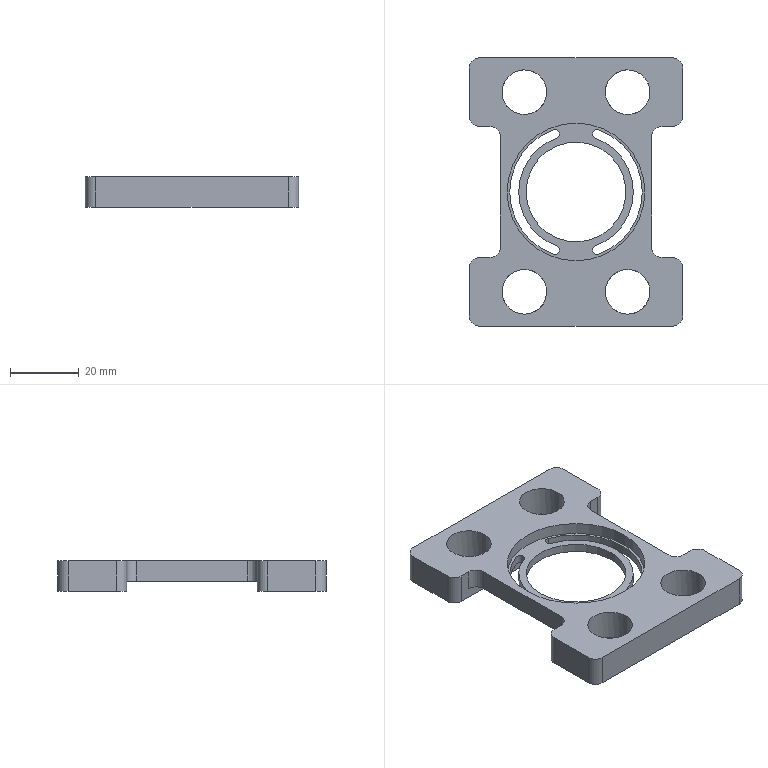NC program | NX | posted with a generic post | part box 62 x 78 x 9 mm
Lines 1 to 792 of 3044:
N10 G17 G21 G94 G90
(FLOOR_WALL , TOOL : D10)
N12 T10 M6
N14 G54
N16 G17 G0 G90 X-49. Y32.997 S9500 M3
N18 G43 Z30. H10
N20 Z3.
N22 G94 G1 Z0. F1250.
N24 X-46.
N26 X46.
N28 Y28.228
N30 X-46.
N32 Y23.459
N34 X46.
N36 Y18.69
N38 X-46.
N40 Y13.921
N42 X46.
N44 Y9.152
N46 X-46.
N48 Y4.383
N50 X46.
N52 Y-0.386
N54 X-46.
N56 Y-5.155
N58 X46.
N60 Y-9.924
N62 X-46.
N64 Y-14.693
N66 X46.
N68 Y-19.462
N70 X-46.
N72 Y-24.231
N74 X46.
N76 Y-29.
N78 X-46.
N80 X-49.
N82 Z3.
N84 G0 Z30.
(HOLE_MILLING , TOOL : D10)
N86 X-29. Y15.
N88 Z0.5
N90 G3 X-29.7 Y14.3 R0.7
N92 X-29. Y13.6 R0.7
N94 X-29. Y13.6 Z0. I0. J1.4
N96 X-29. Y13.6 Z-0.5 I0. J1.4
N98 X-29. Y13.6 Z-1. I0. J1.4
N100 X-29. Y13.6 Z-1.5 I0. J1.4
N102 X-29. Y13.6 Z-2. I0. J1.4
N104 X-29. Y13.6 Z-2.5 I0. J1.4
N106 X-29. Y13.6 Z-3. I0. J1.4
N108 X-29. Y13.6 Z-3.5 I0. J1.4
N110 X-29. Y13.6 Z-4. I0. J1.4
N112 X-29. Y13.6 Z-4.5 I0. J1.4
N114 X-29. Y13.6 Z-5. I0. J1.4
N116 X-29. Y13.6 Z-5.5 I0. J1.4
N118 X-29. Y13.6 Z-6. I0. J1.4
N120 X-29. Y13.6 Z-6.5 I0. J1.4
N122 X-29. Y13.6 Z-7. I0. J1.4
N124 X-29. Y13.6 Z-7.5 I0. J1.4
N126 X-29. Y13.6 Z-8. I0. J1.4
N128 X-29. Y13.6 Z-8.5 I0. J1.4
N130 X-29. Y13.6 Z-9. I0. J1.4
N132 X-27.6 Y15. R1.4
N134 X-29. Y13.6 R-1.4
N136 X-28.3 Y14.3 R0.7
N138 X-29. Y15. R0.7
N140 G0 Z30.
N142 Y-15.
N144 Z0.5
N146 G3 X-29.7 Y-15.7 R0.7
N148 X-29. Y-16.4 R0.7
N150 X-29. Y-16.4 Z0. I0. J1.4
N152 X-29. Y-16.4 Z-0.5 I0. J1.4
N154 X-29. Y-16.4 Z-1. I0. J1.4
N156 X-29. Y-16.4 Z-1.5 I0. J1.4
N158 X-29. Y-16.4 Z-2. I0. J1.4
N160 X-29. Y-16.4 Z-2.5 I0. J1.4
N162 X-29. Y-16.4 Z-3. I0. J1.4
N164 X-29. Y-16.4 Z-3.5 I0. J1.4
N166 X-29. Y-16.4 Z-4. I0. J1.4
N168 X-29. Y-16.4 Z-4.5 I0. J1.4
N170 X-29. Y-16.4 Z-5. I0. J1.4
N172 X-29. Y-16.4 Z-5.5 I0. J1.4
N174 X-29. Y-16.4 Z-6. I0. J1.4
N176 X-29. Y-16.4 Z-6.5 I0. J1.4
N178 X-29. Y-16.4 Z-7. I0. J1.4
N180 X-29. Y-16.4 Z-7.5 I0. J1.4
N182 X-29. Y-16.4 Z-8. I0. J1.4
N184 X-29. Y-16.4 Z-8.5 I0. J1.4
N186 X-29. Y-16.4 Z-9. I0. J1.4
N188 X-27.6 Y-15. R1.4
N190 X-29. Y-16.4 R-1.4
N192 X-28.3 Y-15.7 R0.7
N194 X-29. Y-15. R0.7
N196 G0 Z30.
N198 X29.
N200 Z0.5
N202 G3 X28.3 Y-15.7 R0.7
N204 X29. Y-16.4 R0.7
N206 X29. Y-16.4 Z0. I0. J1.4
N208 X29. Y-16.4 Z-0.5 I0. J1.4
N210 X29. Y-16.4 Z-1. I0. J1.4
N212 X29. Y-16.4 Z-1.5 I0. J1.4
N214 X29. Y-16.4 Z-2. I0. J1.4
N216 X29. Y-16.4 Z-2.5 I0. J1.4
N218 X29. Y-16.4 Z-3. I0. J1.4
N220 X29. Y-16.4 Z-3.5 I0. J1.4
N222 X29. Y-16.4 Z-4. I0. J1.4
N224 X29. Y-16.4 Z-4.5 I0. J1.4
N226 X29. Y-16.4 Z-5. I0. J1.4
N228 X29. Y-16.4 Z-5.5 I0. J1.4
N230 X29. Y-16.4 Z-6. I0. J1.4
N232 X29. Y-16.4 Z-6.5 I0. J1.4
N234 X29. Y-16.4 Z-7. I0. J1.4
N236 X29. Y-16.4 Z-7.5 I0. J1.4
N238 X29. Y-16.4 Z-8. I0. J1.4
N240 X29. Y-16.4 Z-8.5 I0. J1.4
N242 X29. Y-16.4 Z-9. I0. J1.4
N244 X30.4 Y-15. R1.4
N246 X29. Y-16.4 R-1.4
N248 X29.7 Y-15.7 R0.7
N250 X29. Y-15. R0.7
N252 G0 Z30.
N254 Y15.
N256 Z0.5
N258 G3 X28.3 Y14.3 R0.7
N260 X29. Y13.6 R0.7
N262 X29. Y13.6 Z0. I0. J1.4
N264 X29. Y13.6 Z-0.5 I0. J1.4
N266 X29. Y13.6 Z-1. I0. J1.4
N268 X29. Y13.6 Z-1.5 I0. J1.4
N270 X29. Y13.6 Z-2. I0. J1.4
N272 X29. Y13.6 Z-2.5 I0. J1.4
N274 X29. Y13.6 Z-3. I0. J1.4
N276 X29. Y13.6 Z-3.5 I0. J1.4
N278 X29. Y13.6 Z-4. I0. J1.4
N280 X29. Y13.6 Z-4.5 I0. J1.4
N282 X29. Y13.6 Z-5. I0. J1.4
N284 X29. Y13.6 Z-5.5 I0. J1.4
N286 X29. Y13.6 Z-6. I0. J1.4
N288 X29. Y13.6 Z-6.5 I0. J1.4
N290 X29. Y13.6 Z-7. I0. J1.4
N292 X29. Y13.6 Z-7.5 I0. J1.4
N294 X29. Y13.6 Z-8. I0. J1.4
N296 X29. Y13.6 Z-8.5 I0. J1.4
N298 X29. Y13.6 Z-9. I0. J1.4
N300 X30.4 Y15. R1.4
N302 X29. Y13.6 R-1.4
N304 X29.7 Y14.3 R0.7
N306 X29. Y15. R0.7
N308 G0 Z30.
(HOLE_MILLING_COPY , TOOL : D10)
N310 X0. Y0.
N312 Z0.5
N314 G3 X-2.483 Y-2.483 R2.483
N316 X0. Y-4.967 R2.483
N318 X0. Y-4.967 Z0. I0. J4.967
N320 X0. Y-4.967 Z-0.5 I0. J4.967
N322 X0. Y-4.967 Z-1. I0. J4.967
N324 X0. Y-4.967 Z-1.5 I0. J4.967
N326 X0. Y-4.967 Z-2. I0. J4.967
N328 X0. Y-4.967 Z-2.5 I0. J4.967
N330 X0. Y-4.967 Z-3. I0. J4.967
N332 X0. Y-4.967 Z-3.5 I0. J4.967
N334 X4.967 Y0. R4.967
N336 X0. Y-4.967 R-4.967
N338 X2.483 Y-2.483 R2.483
N340 X0. Y0. R2.483
N342 G0 Z0.5
N344 G3 X-4.967 Y-4.967 R4.967
N346 X0. Y-9.933 R4.967
N348 X0. Y-9.933 Z0. I0. J9.933
N350 X0. Y-9.933 Z-0.5 I0. J9.933
N352 X0. Y-9.933 Z-1. I0. J9.933
N354 X0. Y-9.933 Z-1.5 I0. J9.933
N356 X0. Y-9.933 Z-2. I0. J9.933
N358 X0. Y-9.933 Z-2.5 I0. J9.933
N360 X0. Y-9.933 Z-3. I0. J9.933
N362 X0. Y-9.933 Z-3.5 I0. J9.933
N364 X9.933 Y0. R9.933
N366 X0. Y-9.933 R-9.933
N368 X4.967 Y-4.967 R4.967
N370 X0. Y0. R4.967
N372 G0 Z0.5
N374 G3 X-7.45 Y-7.45 R7.45
N376 X0. Y-14.9 R7.45
N378 X0. Y-14.9 Z0. I0. J14.9
N380 X0. Y-14.9 Z-0.5 I0. J14.9
N382 X0. Y-14.9 Z-1. I0. J14.9
N384 X0. Y-14.9 Z-1.5 I0. J14.9
N386 X0. Y-14.9 Z-2. I0. J14.9
N388 X0. Y-14.9 Z-2.5 I0. J14.9
N390 X0. Y-14.9 Z-3. I0. J14.9
N392 X0. Y-14.9 Z-3.5 I0. J14.9
N394 X14.9 Y0. R14.9
N396 X0. Y-14.9 R-14.9
N398 X7.45 Y-7.45 R7.45
N400 X0. Y0. R7.45
N402 G0 Z30.
(HOLE_MILLING_COPY_COPY , TOOL : D10)
N404 Z-3.
N406 G3 X-2.35 Y-2.35 R2.35
N408 X0. Y-4.7 R2.35
N410 X0. Y-4.7 Z-3.5 I0. J4.7
N412 X0. Y-4.7 Z-4. I0. J4.7
N414 X0. Y-4.7 Z-4.5 I0. J4.7
N416 X0. Y-4.7 Z-5. I0. J4.7
N418 X0. Y-4.7 Z-5.5 I0. J4.7
N420 X0. Y-4.7 Z-6. I0. J4.7
N422 X4.7 Y0. R4.7
N424 X0. Y-4.7 R-4.7
N426 X2.35 Y-2.35 R2.35
N428 X0. Y0. R2.35
N430 G0 Z-3.
N432 G3 X-4.7 Y-4.7 R4.7
N434 X0. Y-9.4 R4.7
N436 X0. Y-9.4 Z-3.5 I0. J9.4
N438 X0. Y-9.4 Z-4. I0. J9.4
N440 X0. Y-9.4 Z-4.5 I0. J9.4
N442 X0. Y-9.4 Z-5. I0. J9.4
N444 X0. Y-9.4 Z-5.5 I0. J9.4
N446 X0. Y-9.4 Z-6. I0. J9.4
N448 X9.4 Y0. R9.4
N450 X0. Y-9.4 R-9.4
N452 X4.7 Y-4.7 R4.7
N454 X0. Y0. R4.7
N456 G0 Z30.
N458 M5
(ZLEVEL_PROFILE , TOOL : D6)
N460 T06 M6
N462 G54
N464 G17 G0 G90 X35.551 Y34.1 S9500 M3
N466 G43 Z30. H6
N468 Z1.5
N470 G94 G1 X36.606 Z1.445 F1000.
N472 X38.237 Y33.707 Z1.357
N474 X39.701 Y32.887 Z1.269
N476 X40.887 Y31.701 Z1.181
N478 X41.707 Y30.237 Z1.093
N480 X42.1 Y28.606 Z1.005
N482 Y28. Z0.973
N484 Y0. Z-0.494
N486 Y-28. F2500.
N488 G2 X36. Y-34.1 R6.1
N490 G1 X22.
N492 G2 X15.9 Y-28. R6.1
N494 G1 Y-25.1
N496 X-15.9
N498 Y-28.
N500 G2 X-22. Y-34.1 R6.1
N502 G1 X-36.
N504 G2 X-42.1 Y-28. R6.1
N506 G1 Y28.
N508 G2 X-36. Y34.1 R6.1
N510 G1 X-22.
N512 G2 X-15.9 Y28. R6.1
N514 G1 Y25.1
N516 X15.9
N518 Y28.
N520 G2 X22. Y34.1 R6.1
N522 G1 X36.
N524 G2 X42.1 Y28. R6.1
N526 G1 Y0.
N528 Y-27.718 Z-0.978
N530 Y-28.013 Z-0.983
N532 X42.092 Y-28.308 Z-0.988
N534 G2 X36. Y-34.1 R6.1
N536 G1 X22.
N538 G2 X15.9 Y-28. R6.1
N540 G1 Y-25.1
N542 X-15.9
N544 Y-28.
N546 G2 X-22. Y-34.1 R6.1
N548 G1 X-36.
N550 G2 X-42.1 Y-28. R6.1
N552 G1 Y28.
N554 G2 X-36. Y34.1 R6.1
N556 G1 X-22.
N558 G2 X-15.9 Y28. R6.1
N560 G1 Y25.1
N562 X15.9
N564 Y28.
N566 G2 X22. Y34.1 R6.1
N568 G1 X36.
N570 G2 X42.1 Y28. R6.1
N572 G1 Y0.
N574 Y-27.718 Z-1.472
N576 Y-28.013 Z-1.477
N578 X42.092 Y-28.308 Z-1.482
N580 G2 X36. Y-34.1 R6.1
N582 G1 X22.
N584 G2 X15.9 Y-28. R6.1
N586 G1 Y-25.1
N588 X-15.9
N590 Y-28.
N592 G2 X-22. Y-34.1 R6.1
N594 G1 X-36.
N596 G2 X-42.1 Y-28. R6.1
N598 G1 Y28.
N600 G2 X-36. Y34.1 R6.1
N602 G1 X-22.
N604 G2 X-15.9 Y28. R6.1
N606 G1 Y25.1
N608 X15.9
N610 Y28.
N612 G2 X22. Y34.1 R6.1
N614 G1 X36.
N616 G2 X42.1 Y28. R6.1
N618 G1 Y0.
N620 Y-27.718 Z-1.966
N622 Y-28.013 Z-1.971
N624 X42.092 Y-28.308 Z-1.976
N626 G2 X36. Y-34.1 R6.1
N628 G1 X22.
N630 G2 X15.9 Y-28. R6.1
N632 G1 Y-25.1
N634 X-15.9
N636 Y-28.
N638 G2 X-22. Y-34.1 R6.1
N640 G1 X-36.
N642 G2 X-42.1 Y-28. R6.1
N644 G1 Y28.
N646 G2 X-36. Y34.1 R6.1
N648 G1 X-22.
N650 G2 X-15.9 Y28. R6.1
N652 G1 Y25.1
N654 X15.9
N656 Y28.
N658 G2 X22. Y34.1 R6.1
N660 G1 X36.
N662 G2 X42.1 Y28. R6.1
N664 G1 Y0.
N666 Y-27.718 Z-2.46
N668 Y-28.013 Z-2.465
N670 X42.092 Y-28.308 Z-2.471
N672 G2 X36. Y-34.1 R6.1
N674 G1 X22.
N676 G2 X15.9 Y-28. R6.1
N678 G1 Y-25.1
N680 X-15.9
N682 Y-28.
N684 G2 X-22. Y-34.1 R6.1
N686 G1 X-36.
N688 G2 X-42.1 Y-28. R6.1
N690 G1 Y28.
N692 G2 X-36. Y34.1 R6.1
N694 G1 X-22.
N696 G2 X-15.9 Y28. R6.1
N698 G1 Y25.1
N700 X15.9
N702 Y28.
N704 G2 X22. Y34.1 R6.1
N706 G1 X36.
N708 G2 X42.1 Y28. R6.1
N710 G1 Y0.
N712 Y-27.718 Z-2.954
N714 Y-28.013 Z-2.96
N716 X42.092 Y-28.308 Z-2.965
N718 G2 X36. Y-34.1 R6.1
N720 G1 X22.
N722 G2 X15.9 Y-28. R6.1
N724 G1 Y-25.1
N726 X-15.9
N728 Y-28.
N730 G2 X-22. Y-34.1 R6.1
N732 G1 X-36.
N734 G2 X-42.1 Y-28. R6.1
N736 G1 Y28.
N738 G2 X-36. Y34.1 R6.1
N740 G1 X-22.
N742 G2 X-15.9 Y28. R6.1
N744 G1 Y25.1
N746 X15.9
N748 Y28.
N750 G2 X22. Y34.1 R6.1
N752 G1 X36.
N754 G2 X42.1 Y28. R6.1
N756 G1 Y0.
N758 Y-27.718 Z-3.449
N760 Y-28.013 Z-3.454
N762 X42.092 Y-28.308 Z-3.459
N764 G2 X36. Y-34.1 R6.1
N766 G1 X22.
N768 G2 X15.9 Y-28. R6.1
N770 G1 Y-25.1
N772 X-15.9
N774 Y-28.
N776 G2 X-22. Y-34.1 R6.1
N778 G1 X-36.
N780 G2 X-42.1 Y-28. R6.1
N782 G1 Y28.
N784 G2 X-36. Y34.1 R6.1
N786 G1 X-22.
N788 G2 X-15.9 Y28. R6.1
N790 G1 Y25.1
N792 X15.9
N794 Y28.
N796 G2 X22. Y34.1 R6.1
N798 G1 X36.
N800 G2 X42.1 Y28. R6.1
N802 G1 Y0.
N804 Y-27.718 Z-3.943
N806 Y-28.013 Z-3.948
N808 X42.092 Y-28.308 Z-3.953
N810 G2 X36. Y-34.1 R6.1
N812 G1 X22.
N814 G2 X15.9 Y-28. R6.1
N816 G1 Y-25.1
N818 X-15.9
N820 Y-28.
N822 G2 X-22. Y-34.1 R6.1
N824 G1 X-36.
N826 G2 X-42.1 Y-28. R6.1
N828 G1 Y28.
N830 G2 X-36. Y34.1 R6.1
N832 G1 X-22.
N834 G2 X-15.9 Y28. R6.1
N836 G1 Y25.1
N838 X15.9
N840 Y28.
N842 G2 X22. Y34.1 R6.1
N844 G1 X36.
N846 G2 X42.1 Y28. R6.1
N848 G1 Y0.
N850 Y-27.718 Z-4.437
N852 Y-28.013 Z-4.442
N854 X42.092 Y-28.308 Z-4.447
N856 G2 X36. Y-34.1 R6.1
N858 G1 X22.
N860 G2 X15.9 Y-28. R6.1
N862 G1 Y-25.1
N864 X-15.9
N866 Y-28.
N868 G2 X-22. Y-34.1 R6.1
N870 G1 X-36.
N872 G2 X-42.1 Y-28. R6.1
N874 G1 Y28.
N876 G2 X-36. Y34.1 R6.1
N878 G1 X-22.
N880 G2 X-15.9 Y28. R6.1
N882 G1 Y25.1
N884 X15.9
N886 Y28.
N888 G2 X22. Y34.1 R6.1
N890 G1 X36.
N892 G2 X42.1 Y28. R6.1
N894 G1 Y0.
N896 Y-27.718 Z-4.931
N898 Y-28.013 Z-4.936
N900 X42.092 Y-28.308 Z-4.941
N902 G2 X36. Y-34.1 R6.1
N904 G1 X22.
N906 G2 X15.9 Y-28. R6.1
N908 G1 Y-25.1
N910 X-15.9
N912 Y-28.
N914 G2 X-22. Y-34.1 R6.1
N916 G1 X-36.
N918 G2 X-42.1 Y-28. R6.1
N920 G1 Y28.
N922 G2 X-36. Y34.1 R6.1
N924 G1 X-22.
N926 G2 X-15.9 Y28. R6.1
N928 G1 Y25.1
N930 X15.9
N932 Y28.
N934 G2 X22. Y34.1 R6.1
N936 G1 X36.
N938 G2 X42.1 Y28. R6.1
N940 G1 Y0.
N942 Y-27.718 Z-5.425
N944 Y-28.013 Z-5.43
N946 X42.092 Y-28.308 Z-5.435
N948 G2 X36. Y-34.1 R6.1
N950 G1 X22.
N952 G2 X15.9 Y-28. R6.1
N954 G1 Y-25.1
N956 X-15.9
N958 Y-28.
N960 G2 X-22. Y-34.1 R6.1
N962 G1 X-36.
N964 G2 X-42.1 Y-28. R6.1
N966 G1 Y28.
N968 G2 X-36. Y34.1 R6.1
N970 G1 X-22.
N972 G2 X-15.9 Y28. R6.1
N974 G1 Y25.1
N976 X15.9
N978 Y28.
N980 G2 X22. Y34.1 R6.1
N982 G1 X36.
N984 G2 X42.1 Y28. R6.1
N986 G1 Y0.
N988 Y-27.718 Z-5.919
N990 Y-28.013 Z-5.924
N992 X42.092 Y-28.308 Z-5.929
N994 G2 X36. Y-34.1 R6.1
N996 G1 X22.
N998 G2 X15.9 Y-28. R6.1
N1000 G1 Y-25.1
N1002 X-15.9
N1004 Y-28.
N1006 G2 X-22. Y-34.1 R6.1
N1008 G1 X-36.
N1010 G2 X-42.1 Y-28. R6.1
N1012 G1 Y28.
N1014 G2 X-36. Y34.1 R6.1
N1016 G1 X-22.
N1018 G2 X-15.9 Y28. R6.1
N1020 G1 Y25.1
N1022 X15.9
N1024 Y28.
N1026 G2 X22. Y34.1 R6.1
N1028 G1 X36.
N1030 G2 X42.1 Y28. R6.1
N1032 G1 Y0.
N1034 Y-27.718 Z-6.413
N1036 Y-28.013 Z-6.418
N1038 X42.092 Y-28.308 Z-6.424
N1040 G2 X36. Y-34.1 R6.1
N1042 G1 X22.
N1044 G2 X15.9 Y-28. R6.1
N1046 G1 Y-25.1
N1048 X-15.9
N1050 Y-28.
N1052 G2 X-22. Y-34.1 R6.1
N1054 G1 X-36.
N1056 G2 X-42.1 Y-28. R6.1
N1058 G1 Y28.
N1060 G2 X-36. Y34.1 R6.1
N1062 G1 X-22.
N1064 G2 X-15.9 Y28. R6.1
N1066 G1 Y25.1
N1068 X15.9
N1070 Y28.
N1072 G2 X22. Y34.1 R6.1
N1074 G1 X36.
N1076 G2 X42.1 Y28. R6.1
N1078 G1 Y0.
N1080 Y-27.718 Z-6.907
N1082 Y-28.013 Z-6.913
N1084 X42.092 Y-28.308 Z-6.918
N1086 G2 X36. Y-34.1 R6.1
N1088 G1 X22.
N1090 G2 X15.9 Y-28. R6.1
N1092 G1 Y-25.1
N1094 X-15.9
N1096 Y-28.
N1098 G2 X-22. Y-34.1 R6.1
N1100 G1 X-36.
N1102 G2 X-42.1 Y-28. R6.1
N1104 G1 Y28.
N1106 G2 X-36. Y34.1 R6.1
N1108 G1 X-22.
N1110 G2 X-15.9 Y28. R6.1
N1112 G1 Y25.1
N1114 X15.9
N1116 Y28.
N1118 G2 X22. Y34.1 R6.1
N1120 G1 X36.
N1122 G2 X42.1 Y28. R6.1
N1124 G1 Y0.
N1126 Y-27.718 Z-7.401
N1128 Y-28.013 Z-7.407
N1130 X42.092 Y-28.308 Z-7.412
N1132 G2 X36. Y-34.1 R6.1
N1134 G1 X22.
N1136 G2 X15.9 Y-28. R6.1
N1138 G1 Y-25.1
N1140 X-15.9
N1142 Y-28.
N1144 G2 X-22. Y-34.1 R6.1
N1146 G1 X-36.
N1148 G2 X-42.1 Y-28. R6.1
N1150 G1 Y28.
N1152 G2 X-36. Y34.1 R6.1
N1154 G1 X-22.
N1156 G2 X-15.9 Y28. R6.1
N1158 G1 Y25.1
N1160 X15.9
N1162 Y28.
N1164 G2 X22. Y34.1 R6.1
N1166 G1 X36.
N1168 G2 X42.1 Y28. R6.1
N1170 G1 Y0.
N1172 Y-27.718 Z-7.896
N1174 Y-28.013 Z-7.901
N1176 X42.092 Y-28.308 Z-7.906
N1178 G2 X36. Y-34.1 R6.1
N1180 G1 X22.
N1182 G2 X15.9 Y-28. R6.1
N1184 G1 Y-25.1
N1186 X-15.9
N1188 Y-28.
N1190 G2 X-22. Y-34.1 R6.1
N1192 G1 X-36.
N1194 G2 X-42.1 Y-28. R6.1
N1196 G1 Y28.
N1198 G2 X-36. Y34.1 R6.1
N1200 G1 X-22.
N1202 G2 X-15.9 Y28. R6.1
N1204 G1 Y25.1
N1206 X15.9
N1208 Y28.
N1210 G2 X22. Y34.1 R6.1
N1212 G1 X36.
N1214 G2 X42.1 Y28. R6.1
N1216 G1 Y0.
N1218 Y-27.718 Z-8.39
N1220 Y-28.013 Z-8.395
N1222 X42.092 Y-28.308 Z-8.4
N1224 G2 X36. Y-34.1 R6.1
N1226 G1 X22.
N1228 G2 X15.9 Y-28. R6.1
N1230 G1 Y-25.1
N1232 X-15.9
N1234 Y-28.
N1236 G2 X-22. Y-34.1 R6.1
N1238 G1 X-36.
N1240 G2 X-42.1 Y-28. R6.1
N1242 G1 Y28.
N1244 G2 X-36. Y34.1 R6.1
N1246 G1 X-22.
N1248 G2 X-15.9 Y28. R6.1
N1250 G1 Y25.1
N1252 X15.9
N1254 Y28.
N1256 G2 X22. Y34.1 R6.1
N1258 G1 X36.
N1260 G2 X42.1 Y28. R6.1
N1262 G1 Y-28.
N1264 G2 X42.092 Y-28.308 R6.1
N1266 G1 Z-6.9
N1268 G0 Z30.
(ZLEVEL_PROFILE_COPY , TOOL : D6)
N1270 X31.278 Y-15.319
N1272 Z-2.5
N1274 G1 Z-3.5 F1000.
N1276 X32.286 Y-15.46
N1278 G3 X32.5 Y-15. R0.6
N1280 X29. Y-11.5 R3.5
N1282 X32.5 Y-15. R-3.5
N1284 X32.286 Y-14.54 R0.6
N1286 G1 X31.278 Y-14.681
N1288 Z-2.5
N1290 G0 Z30.
N1292 Y-15.319
N1294 Z-8.
N1296 G1 Z-9.
N1298 X32.286 Y-15.46
N1300 G3 X32.5 Y-15. R0.6
N1302 X29. Y-11.5 R3.5
N1304 X32.5 Y-15. R-3.5
N1306 X32.286 Y-14.54 R0.6
N1308 G1 X31.278 Y-14.681
N1310 Z-8.
N1312 G0 Z30.
N1314 X-1.334 Y-15.744
N1316 Z-2.5
N1318 G1 Z-3.5
N1320 X-0.46 Y-16.786
N1322 G3 X0. Y-17. R0.6
N1324 X17. Y0. R17.
N1326 X0. Y-17. R-17.
N1328 X0.46 Y-16.786 R0.6
N1330 G1 X1.334 Y-15.744
N1332 Z-2.5
N1334 G0 Z30.
N1336 X31.278 Y14.681
N1338 Z-2.5
N1340 G1 Z-3.5
N1342 X32.286 Y14.54
N1344 G3 X32.5 Y15. R0.6
N1346 X29. Y18.5 R3.5
N1348 X32.5 Y15. R-3.5
N1350 X32.286 Y15.46 R0.6
N1352 G1 X31.278 Y15.319
N1354 Z-2.5
N1356 G0 Z30.
N1358 Y14.681
N1360 Z-8.
N1362 G1 Z-9.
N1364 X32.286 Y14.54
N1366 G3 X32.5 Y15. R0.6
N1368 X29. Y18.5 R3.5
N1370 X32.5 Y15. R-3.5
N1372 X32.286 Y15.46 R0.6
N1374 G1 X31.278 Y15.319
N1376 Z-8.
N1378 G0 Z30.
N1380 X-31.278 Y-14.681
N1382 Z-2.5
N1384 G1 Z-3.5
N1386 X-32.286 Y-14.54
N1388 G3 X-32.5 Y-15. R0.6
N1390 X-29. Y-18.5 R3.5
N1392 X-32.5 Y-15. R-3.5
N1394 X-32.286 Y-15.46 R0.6
N1396 G1 X-31.278 Y-15.319
N1398 Z-2.5
N1400 G0 Z30.
N1402 Y-14.681
N1404 Z-8.
N1406 G1 Z-9.
N1408 X-32.286 Y-14.54
N1410 G3 X-32.5 Y-15. R0.6
N1412 X-29. Y-18.5 R3.5
N1414 X-32.5 Y-15. R-3.5
N1416 X-32.286 Y-15.46 R0.6
N1418 G1 X-31.278 Y-15.319
N1420 Z-8.
N1422 G0 Z30.
N1424 Y15.319
N1426 Z-2.5
N1428 G1 Z-3.5
N1430 X-32.286 Y15.46
N1432 G3 X-32.5 Y15. R0.6
N1434 X-29. Y11.5 R3.5
N1436 X-32.5 Y15. R-3.5
N1438 X-32.286 Y14.54 R0.6
N1440 G1 X-31.278 Y14.681
N1442 Z-2.5
N1444 G0 Z30.
N1446 Y15.319
N1448 Z-8.
N1450 G1 Z-9.
N1452 X-32.286 Y15.46
N1454 G3 X-32.5 Y15. R0.6
N1456 X-29. Y11.5 R3.5
N1458 X-32.5 Y15. R-3.5
N1460 X-32.286 Y14.54 R0.6
N1462 G1 X-31.278 Y14.681
N1464 Z-8.
N1466 G0 Z30.
(ZLEVEL_PROFILE_COPY_COPY , TOOL : D6)
N1468 X-4.346 Y9.338
N1470 Z-5.
N1472 G1 Z-6.
N1474 X-5.686 Y9.759
N1476 G3 X-6.189 Y9.693 R0.6
N1478 X-8.344 Y7.914 R11.5
N1480 G1 X-8.501 Y7.745
N1482 G3 X-9.436 Y6.573 R11.5
N1484 G1 X-9.425 Y6.544
N1486 X-9.544 Y6.416
N1488 G3 X-9.012 Y-7.144 R11.5
N1490 G1 X-8.981 Y-7.138
N1492 X-8.939 Y-7.234
N1494 G3 X8.939 Y-7.234 R11.5
N1496 G1 X8.981 Y-7.138
N1498 X9.012 Y-7.144
N1500 G3 X11.327 Y-1.985 R11.5
N1502 G1 X11.302 Y-1.961
N1504 X11.334 Y-1.948
N1506 G3 X9.544 Y6.416 R11.5
N1508 G1 X9.425 Y6.544
N1510 X9.436 Y6.573
N1512 G3 X8.501 Y7.745 R11.5
N1514 G1 X8.344 Y7.914
N1516 G3 X4.208 Y10.703 R11.5
N1518 G1 X4.155 Y10.708
N1520 X3.594 Y10.895
N1522 X3.577 Y10.93
N1524 G3 X1.993 Y11.326 R11.5
N1526 G1 X1.97 Y11.302
N1528 X1.955 Y11.333
N1530 G3 X-1.955 Y11.333 R11.5
N1532 G1 X-1.97 Y11.302
N1534 X-1.993 Y11.326
N1536 G3 X-6.189 Y9.693 R11.5
N1538 X-6.461 Y9.265 R0.6
N1540 G1 X-6.643 Y7.872
N1542 Z-5.
N1544 G0 Z30.
N1546 M5